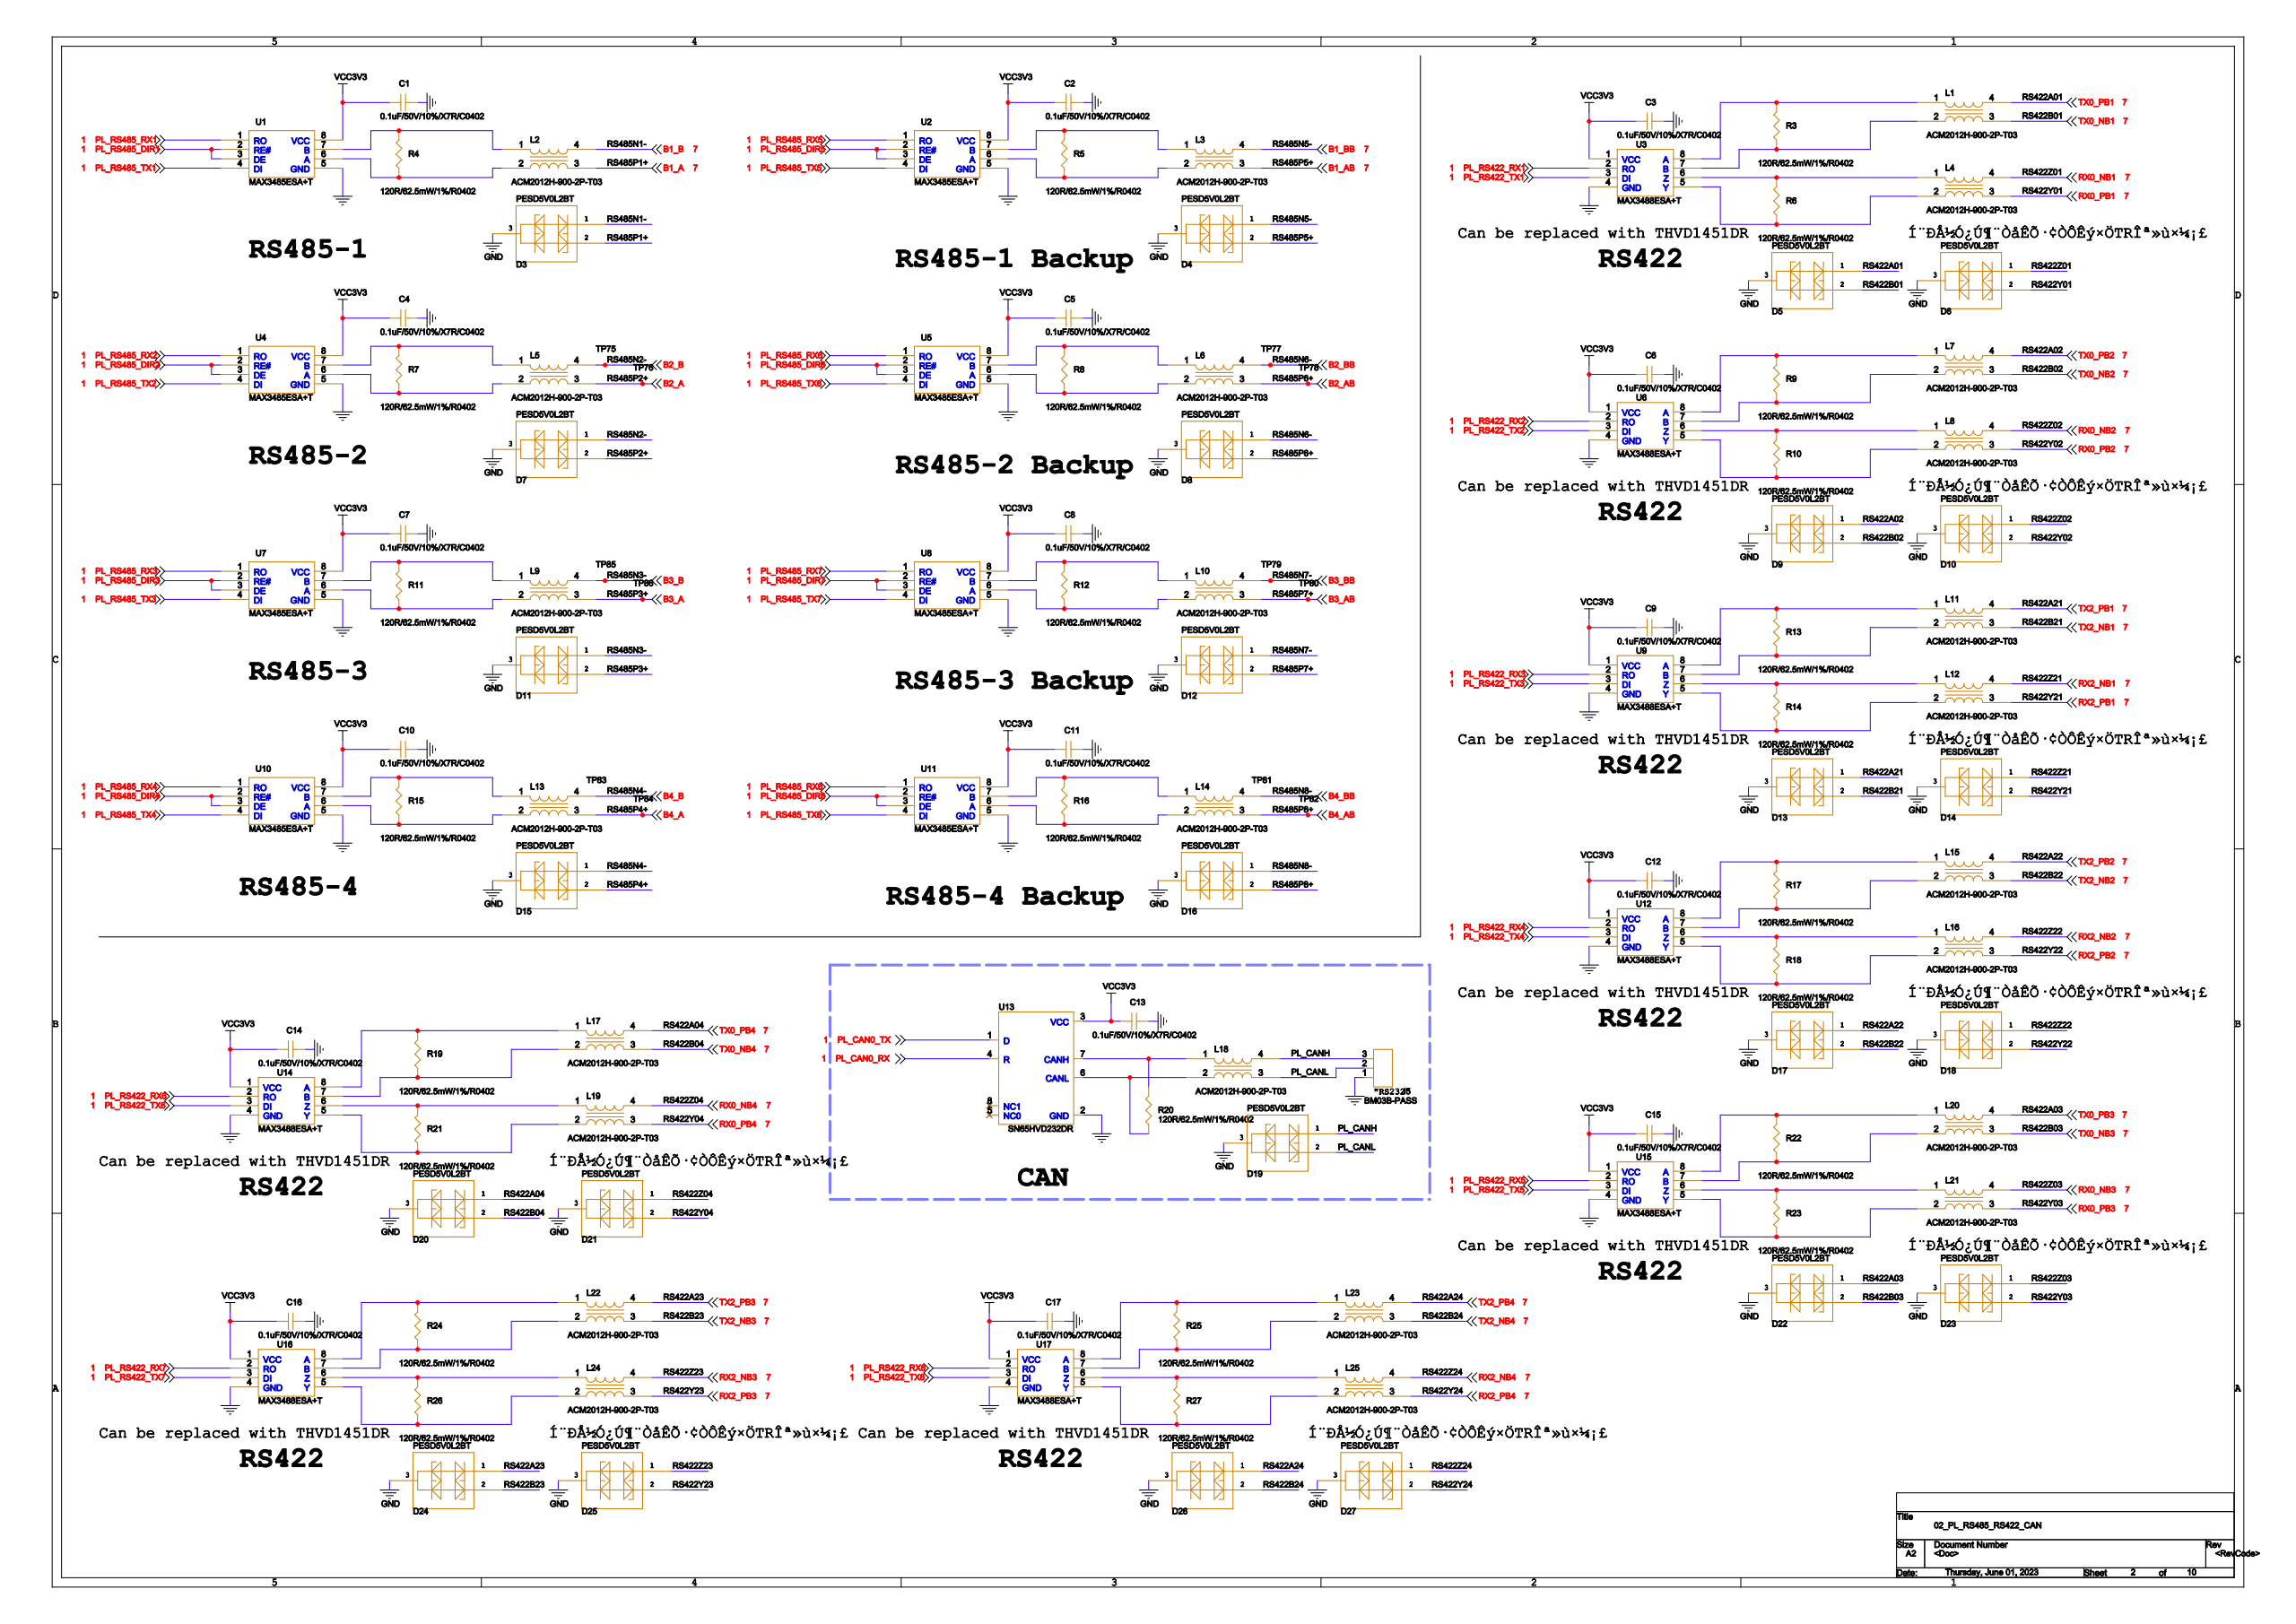Circuit board | Cadence Allegro | 480 parts | 625 nets | one sheet of the schematic
Parts on this sheet (reference | value | footprint):
C1 | 0.1uF/50V/10%/X7R/C0402 | 0402
C2 | 0.1uF/50V/10%/X7R/C0402 | 0402
C3 | 0.1uF/50V/10%/X7R/C0402 | 0402
C4 | 0.1uF/50V/10%/X7R/C0402 | 0402
C5 | 0.1uF/50V/10%/X7R/C0402 | 0402
C6 | 0.1uF/50V/10%/X7R/C0402 | 0402
C7 | 0.1uF/50V/10%/X7R/C0402 | 0402
C8 | 0.1uF/50V/10%/X7R/C0402 | 0402
C9 | 0.1uF/50V/10%/X7R/C0402 | 0402
C10 | 0.1uF/50V/10%/X7R/C0402 | 0402
C11 | 0.1uF/50V/10%/X7R/C0402 | 0402
C12 | 0.1uF/50V/10%/X7R/C0402 | 0402
C13 | 0.1uF/50V/10%/X7R/C0402 | 0402
C14 | 0.1uF/50V/10%/X7R/C0402 | 0402
C15 | 0.1uF/50V/10%/X7R/C0402 | 0402
C16 | 0.1uF/50V/10%/X7R/C0402 | 0402
C17 | 0.1uF/50V/10%/X7R/C0402 | 0402
D3 | PESD5V0L2BT | SOT23
D4 | PESD5V0L2BT | SOT23
D5 | PESD5V0L2BT | SOT23
D6 | PESD5V0L2BT | SOT23
D7 | PESD5V0L2BT | SOT23
D8 | PESD5V0L2BT | SOT23
D9 | PESD5V0L2BT | SOT23
D10 | PESD5V0L2BT | SOT23
D11 | PESD5V0L2BT | SOT23
D12 | PESD5V0L2BT | SOT23
D13 | PESD5V0L2BT | SOT23
D14 | PESD5V0L2BT | SOT23
D15 | PESD5V0L2BT | SOT23
D16 | PESD5V0L2BT | SOT23
D17 | PESD5V0L2BT | SOT23
D18 | PESD5V0L2BT | SOT23
D19 | PESD5V0L2BT | SOT23
D20 | PESD5V0L2BT | SOT23
D21 | PESD5V0L2BT | SOT23
D22 | PESD5V0L2BT | SOT23
D23 | PESD5V0L2BT | SOT23
D24 | PESD5V0L2BT | SOT23
D25 | PESD5V0L2BT | SOT23
D26 | PESD5V0L2BT | SOT23
D27 | PESD5V0L2BT | SOT23
J5 | BM03B-PASS | JK2EDGRC-381-3_S
L1 | ACM2012H-900-2P-T03 | ACM2012
L2 | ACM2012H-900-2P-T03 | ACM2012
L3 | ACM2012H-900-2P-T03 | ACM2012
L4 | ACM2012H-900-2P-T03 | ACM2012
L5 | ACM2012H-900-2P-T03 | ACM2012
L6 | ACM2012H-900-2P-T03 | ACM2012
L7 | ACM2012H-900-2P-T03 | ACM2012
L8 | ACM2012H-900-2P-T03 | ACM2012
L9 | ACM2012H-900-2P-T03 | ACM2012
L10 | ACM2012H-900-2P-T03 | ACM2012
L11 | ACM2012H-900-2P-T03 | ACM2012
L12 | ACM2012H-900-2P-T03 | ACM2012
L13 | ACM2012H-900-2P-T03 | ACM2012
L14 | ACM2012H-900-2P-T03 | ACM2012
L15 | ACM2012H-900-2P-T03 | ACM2012
L16 | ACM2012H-900-2P-T03 | ACM2012
L17 | ACM2012H-900-2P-T03 | ACM2012
L18 | ACM2012H-900-2P-T03 | ACM2012
L19 | ACM2012H-900-2P-T03 | ACM2012
L20 | ACM2012H-900-2P-T03 | ACM2012
L21 | ACM2012H-900-2P-T03 | ACM2012
L22 | ACM2012H-900-2P-T03 | ACM2012
L23 | ACM2012H-900-2P-T03 | ACM2012
L24 | ACM2012H-900-2P-T03 | ACM2012
L25 | ACM2012H-900-2P-T03 | ACM2012
R3 | 120R/62.5mW/1%/R0402 | 0402
R4 | 120R/62.5mW/1%/R0402 | 0402
R5 | 120R/62.5mW/1%/R0402 | 0402
R6 | 120R/62.5mW/1%/R0402 | 0402
R7 | 120R/62.5mW/1%/R0402 | 0402
R8 | 120R/62.5mW/1%/R0402 | 0402
R9 | 120R/62.5mW/1%/R0402 | 0402
R10 | 120R/62.5mW/1%/R0402 | 0402
R11 | 120R/62.5mW/1%/R0402 | 0402
R12 | 120R/62.5mW/1%/R0402 | 0402
R13 | 120R/62.5mW/1%/R0402 | 0402
R14 | 120R/62.5mW/1%/R0402 | 0402
R15 | 120R/62.5mW/1%/R0402 | 0402
R16 | 120R/62.5mW/1%/R0402 | 0402
R17 | 120R/62.5mW/1%/R0402 | 0402
R18 | 120R/62.5mW/1%/R0402 | 0402
R19 | 120R/62.5mW/1%/R0402 | 0402
R20 | 120R/62.5mW/1%/R0402 | 0402
R21 | 120R/62.5mW/1%/R0402 | 0402
R22 | 120R/62.5mW/1%/R0402 | 0402
R23 | 120R/62.5mW/1%/R0402 | 0402
R24 | 120R/62.5mW/1%/R0402 | 0402
R25 | 120R/62.5mW/1%/R0402 | 0402
R26 | 120R/62.5mW/1%/R0402 | 0402
R27 | 120R/62.5mW/1%/R0402 | 0402
TP75 | TEST POINT A | TEST_12MM
TP76 | TEST POINT A | TEST_12MM
TP77 | TEST POINT A | TEST_12MM
TP78 | TEST POINT A | TEST_12MM
TP79 | TEST POINT A | TEST_12MM
TP80 | TEST POINT A | TEST_12MM
TP81 | TEST POINT A | TEST_12MM
TP82 | TEST POINT A | TEST_12MM
TP83 | TEST POINT A | TEST_12MM
TP84 | TEST POINT A | TEST_12MM
TP85 | TEST POINT A | TEST_12MM
TP86 | TEST POINT A | TEST_12MM
U1 | MAX3485ESA+T | SO8
U2 | MAX3485ESA+T | SO8
U3 | MAX3488ESA+T | SO8
U4 | MAX3485ESA+T | SO8
U5 | MAX3485ESA+T | SO8
U6 | MAX3488ESA+T | SO8
U7 | MAX3485ESA+T | SO8
U8 | MAX3485ESA+T | SO8
U9 | MAX3488ESA+T | SO8
U10 | MAX3485ESA+T | SO8
U11 | MAX3485ESA+T | SO8
U12 | MAX3488ESA+T | SO8
U13 | SN65HVD232DR | SO8
U14 | MAX3488ESA+T | SO8
U15 | MAX3488ESA+T | SO8
U16 | MAX3488ESA+T | SO8
U17 | MAX3488ESA+T | SO8
Nets of these parts (net: part-pin ...):
AGND: C1-2 C2-2 C3-2 C4-2 C5-2 C6-2 C7-2 C8-2 C9-2 C10-2 C11-2 C12-2 C13-2 C14-2 C15-2 C16-2 C17-2 D3-3 D4-3 D5-3 D6-3 D7-3 D8-3 D9-3 D10-3 D11-3 D12-3 D13-3 D14-3 D15-3 D16-3 D17-3 D18-3 D19-3 D20-3 D21-3 D22-3 D23-3 D24-3 D25-3 D26-3 D27-3 J5-1 U1-5 U2-5 U3-4 U4-5 U5-5 U6-4 U7-5 U8-5 U9-4 U10-5 U11-5 U12-4 U13-2 U14-4 U15-4 U16-4 U17-4
3.3V: C1-1 C2-1 C3-1 C4-1 C5-1 C6-1 C7-1 C8-1 C9-1 C10-1 C11-1 C12-1 C13-1 C14-1 C15-1 C16-1 C17-1 U1-8 U2-8 U3-1 U4-8 U5-8 U6-1 U7-8 U8-8 U9-1 U10-8 U11-8 U12-1 U13-3 U14-1 U15-1 U16-1 U17-1
PL_RS485_DIR3: U7-2 U7-3
PL_RS485_TX2: U4-4
PL_RS485_TX7: U8-4
PL_RS485_DIR2: U4-2 U4-3
PL_RS485_RX7: U8-1
PL_RS485_RX2: U4-1
PL_RS485_TX6: U5-4
PL_RS485_DIR6: U5-2 U5-3
PL_RS485_RX6: U5-1
PL_RS485_TX1: U1-4
PL_RS485_DIR1: U1-2 U1-3
PL_RS485_RX1: U1-1
PL_RS485_DIR5: U2-2 U2-3
PL_RS485_TX5: U2-4
PL_RS485_RX5: U2-1
PL_RS422_TX6: U14-3
PL_RS422_RX1: U3-2
PL_RS422_RX6: U14-2
PL_RS422_TX1: U3-3
PL_RS422_TX8: U17-3
PL_RS422_RX3: U9-2
PL_RS422_RX8: U17-2
PL_RS422_TX3: U9-3
PL_RS422_TX7: U16-3
PL_RS422_RX2: U6-2
PL_RS422_RX7: U16-2
PL_RS422_TX2: U6-3
PL_RS422_TX4: U12-3
PL_RS422_RX5: U15-2
PL_RS422_RX4: U12-2
PL_RS422_TX5: U15-3
PL_CAN0_RX: U13-4
PL_CAN0_TX: U13-1
PL_RS485_DIR8: U11-2 U11-3
PL_RS485_TX4: U10-4
PL_RS485_RX8: U11-1
PL_RS485_DIR4: U10-2 U10-3
PL_RS485_TX3: U7-4
PL_RS485_RX4: U10-1
PL_RS485_RX3: U7-1
PL_RS485_TX8: U11-4
PL_RS485_DIR7: U8-2 U8-3
B1_A: D3-2 L2-3
B1_B: D3-1 L2-4
B1_AB: D4-2 L3-3
B1_BB: D4-1 L3-4
TX0_PB1: D5-1 L1-4
TX0_NB1: D5-2 L1-3
RX0_PB1: D6-2 L4-3
RX0_NB1: D6-1 L4-4
TX2_PB1: D13-1 L11-4
TX2_NB1: D13-2 L11-3
RX2_PB1: D14-2 L12-3
RX2_NB1: D14-1 L12-4
TX0_PB2: D9-1 L7-4
TX0_NB2: D9-2 L7-3
RX0_PB2: D10-2 L8-3
RX0_NB2: D10-1 L8-4
TX2_PB2: D17-1 L15-4
TX2_NB2: D17-2 L15-3
RX2_PB2: D18-2 L16-3
RX2_NB2: D18-1 L16-4
TX2_PB3: D24-1 L22-4
TX2_NB3: D24-2 L22-3
RX2_PB3: D25-2 L24-3
RX2_NB3: D25-1 L24-4
TX0_PB4: D20-1 L17-4
TX0_NB4: D20-2 L17-3
RX0_PB4: D21-2 L19-3
RX0_NB4: D21-1 L19-4
TX2_PB4: D26-1 L23-4
TX2_NB4: D26-2 L23-3
RX2_PB4: D27-2 L25-3
RX2_NB4: D27-1 L25-4
TX0_PB3: D22-1 L20-4
TX0_NB3: D22-2 L20-3
RX0_PB3: D23-2 L21-3
RX0_NB3: D23-1 L21-4
B3_B: D11-1 L9-4 TP85-1
B3_A: D11-2 L9-3 TP86-1
B3_BB: D12-1 L10-4 TP79-1
B3_AB: D12-2 L10-3 TP80-1
B4_B: D15-1 L13-4 TP83-1
B4_A: D15-2 L13-3 TP84-1
B4_BB: D16-1 L14-4 TP81-1
B4_AB: D16-2 L14-3 TP82-1
PL_CANH: D19-1 J5-3 L18-4
PL_CANL: D19-2 J5-2 L18-3
B2_B: D7-1 L5-4 TP75-1
B2_A: D7-2 L5-3 TP76-1
B2_BB: D8-1 L6-4 TP77-1
B2_AB: D8-2 L6-3 TP78-1
N21787149: L1-1 R3-1 U3-8
N21787168: L1-2 R3-2 U3-7
N23301710: L10-1 R12-1 U8-7
N23301716: L10-2 R12-2 U8-6
N23306863: L11-1 R13-1 U9-8
N23306875: L11-2 R13-2 U9-7
N23306883: L12-1 R14-1 U9-6
N23306887: L12-2 R14-2 U9-5
N23302088: L13-1 R15-1 U10-7
N23302102: L13-2 R15-2 U10-6
N23301916: L14-1 R16-1 U11-7
N23301922: L14-2 R16-2 U11-6
N23307430: L15-1 R17-1 U12-8
N23307442: L15-2 R17-2 U12-7
N23307450: L16-1 R18-1 U12-6
N23307454: L16-2 R18-2 U12-5
N23308775: L17-1 R19-1 U14-8
N23308787: L17-2 R19-2 U14-7
N21785912: L18-1 R20-1 U13-7
N21785921: L18-2 R20-2 U13-6
N23308795: L19-1 R21-1 U14-6
N23308799: L19-2 R21-2 U14-5
N21786207: L2-1 R4-1 U1-7
N21786216: L2-2 R4-2 U1-6
N23308016: L20-1 R22-1 U15-8
N23308028: L20-2 R22-2 U15-7
N23308036: L21-1 R23-1 U15-6
N23308040: L21-2 R23-2 U15-5
N23309399: L22-1 R24-1 U16-8
N23309411: L22-2 R24-2 U16-7
N23310458: L23-1 R25-1 U17-8
N23310470: L23-2 R25-2 U17-7
N23309419: L24-1 R26-1 U16-6
N23309423: L24-2 R26-2 U16-5
N23310478: L25-1 R27-1 U17-6
N23310482: L25-2 R27-2 U17-5
N23300009: L3-1 R5-1 U2-7
N23300015: L3-2 R5-2 U2-6
N21787206: L4-1 R6-1 U3-6
N21787225: L4-2 R6-2 U3-5
N23300843: L5-1 R7-1 U4-7
N23300849: L5-2 R7-2 U4-6
N23300689: L6-1 R8-1 U5-7
N23300695: L6-2 R8-2 U5-6
N23306313: L7-1 R9-1 U6-8
N23306325: L7-2 R9-2 U6-7
N23306333: L8-1 R10-1 U6-6
N23306337: L8-2 R10-2 U6-5
N23301864: L9-1 R11-1 U7-7
N23301870: L9-2 R11-2 U7-6